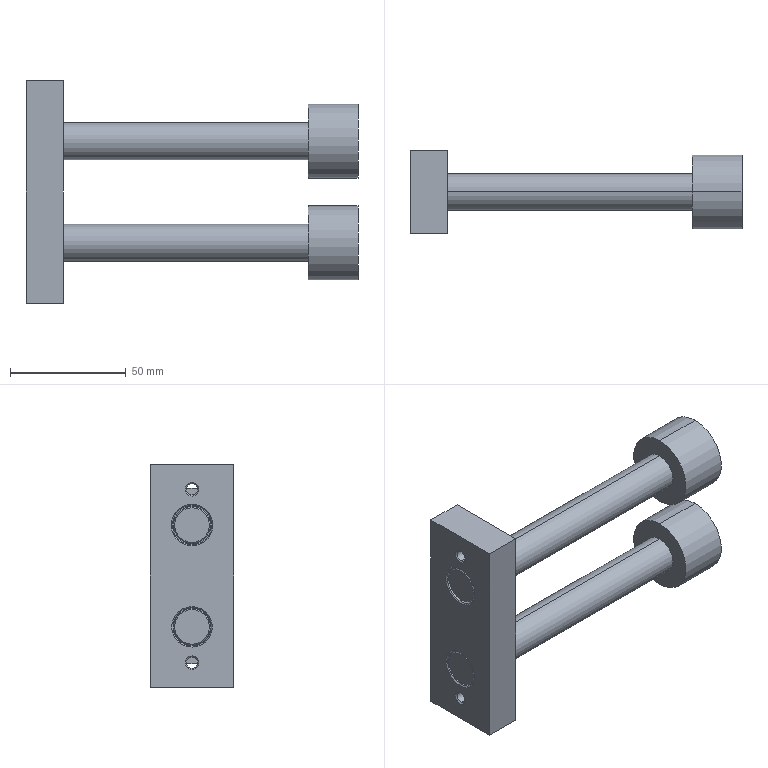Part | SolidWorks | features BaseBody 1 | 1 solid | 67 faces | box 143.5 x 36 x 96 mm | volume 131275 mm3 | cylinder 26 | cone 26 | plane 15 | commonest cylinder face diameters 16 x8 4.134 x4 4.917 x4 32 x4 10 x2 16.5 x2